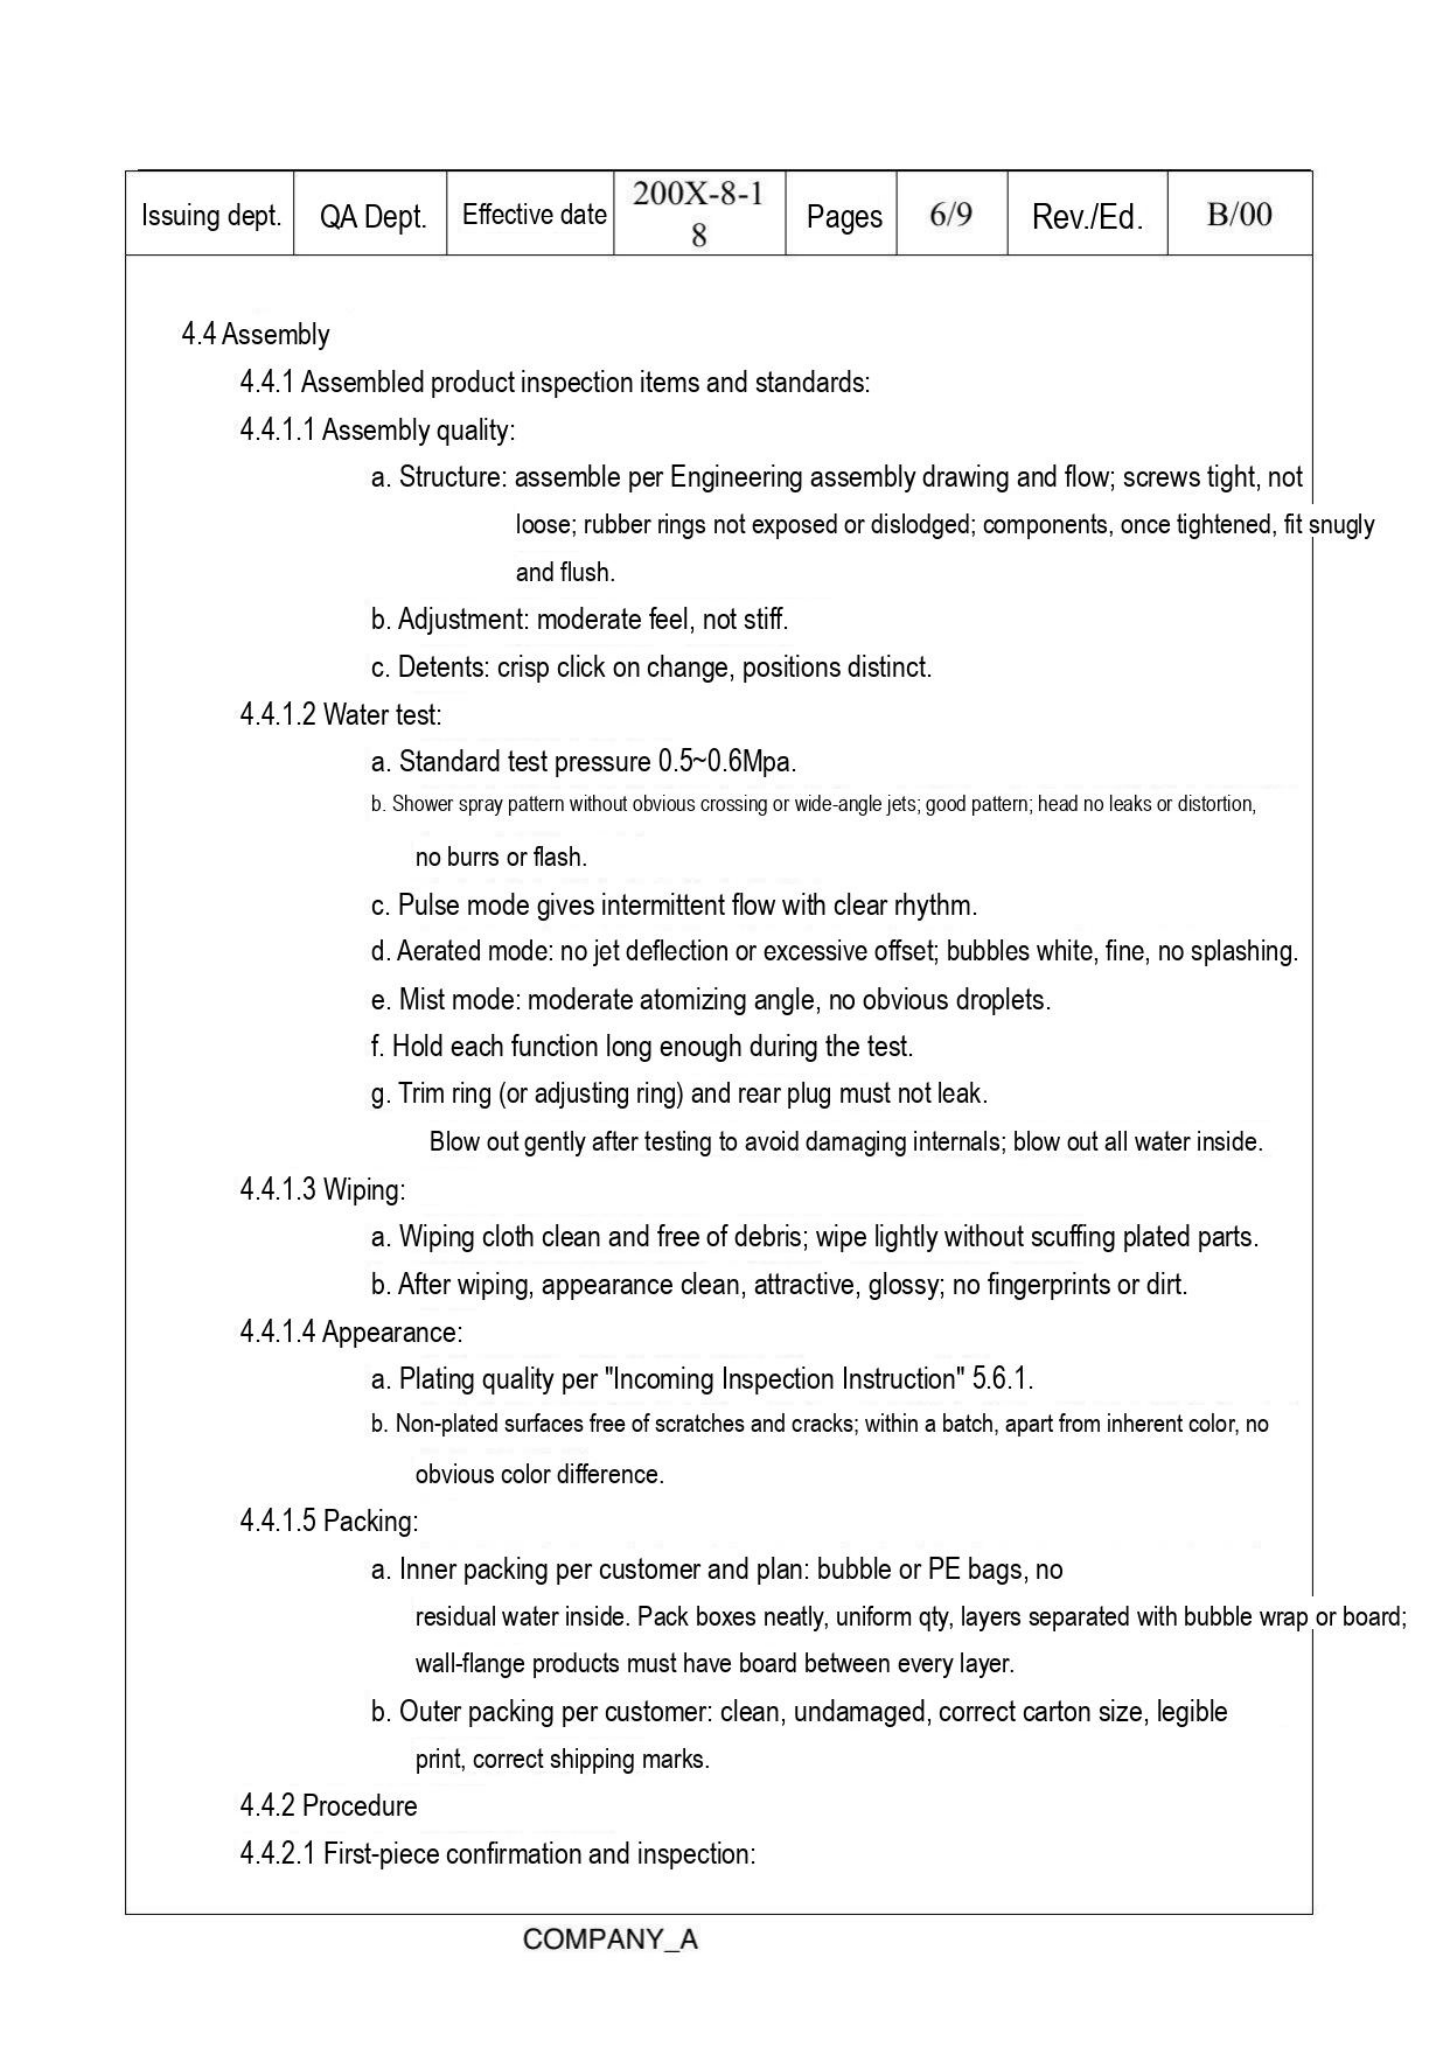| Issuing dept. | QA Dept. | Effective date | 200X-8-18 | Pages | 6/9 | Rev./Ed. | B/00 |
|---|---|---|---|---|---|---|---|

4.4 Assembly

4.4.1 Assembled product inspection items and standards:

4.4.1.1 Assembly quality:

a. Structure: assemble per Engineering assembly drawing and flow; screws tight, not loose; rubber rings not exposed or dislodged; components, once tightened, fit snugly and flush.

b. Adjustment: moderate feel, not stiff.

c. Detents: crisp click on change, positions distinct.

4.4.1.2 Water test:

a. Standard test pressure 0.5~0.6Mpa.

b. Shower spray pattern without obvious crossing or wide-angle jets; good pattern; head no leaks or distortion, no burrs or flash.

c. Pulse mode gives intermittent flow with clear rhythm.

d. Aerated mode: no jet deflection or excessive offset; bubbles white, fine, no splashing.

e. Mist mode: moderate atomizing angle, no obvious droplets.

f. Hold each function long enough during the test.

g. Trim ring (or adjusting ring) and rear plug must not leak.

Blow out gently after testing to avoid damaging internals; blow out all water inside.

4.4.1.3 Wiping:

a. Wiping cloth clean and free of debris; wipe lightly without scuffing plated parts.

b. After wiping, appearance clean, attractive, glossy; no fingerprints or dirt.

4.4.1.4 Appearance:

a. Plating quality per "Incoming Inspection Instruction" 5.6.1.

b. Non-plated surfaces free of scratches and cracks; within a batch, apart from inherent color, no obvious color difference.

4.4.1.5 Packing:

a. Inner packing per customer and plan: bubble or PE bags, no residual water inside. Pack boxes neatly, uniform qty, layers separated with bubble wrap or board; wall-flange products must have board between every layer.

b. Outer packing per customer: clean, undamaged, correct carton size, legible print, correct shipping marks.

4.4.2 Procedure

4.4.2.1 First-piece confirmation and inspection:

COMPANY_A
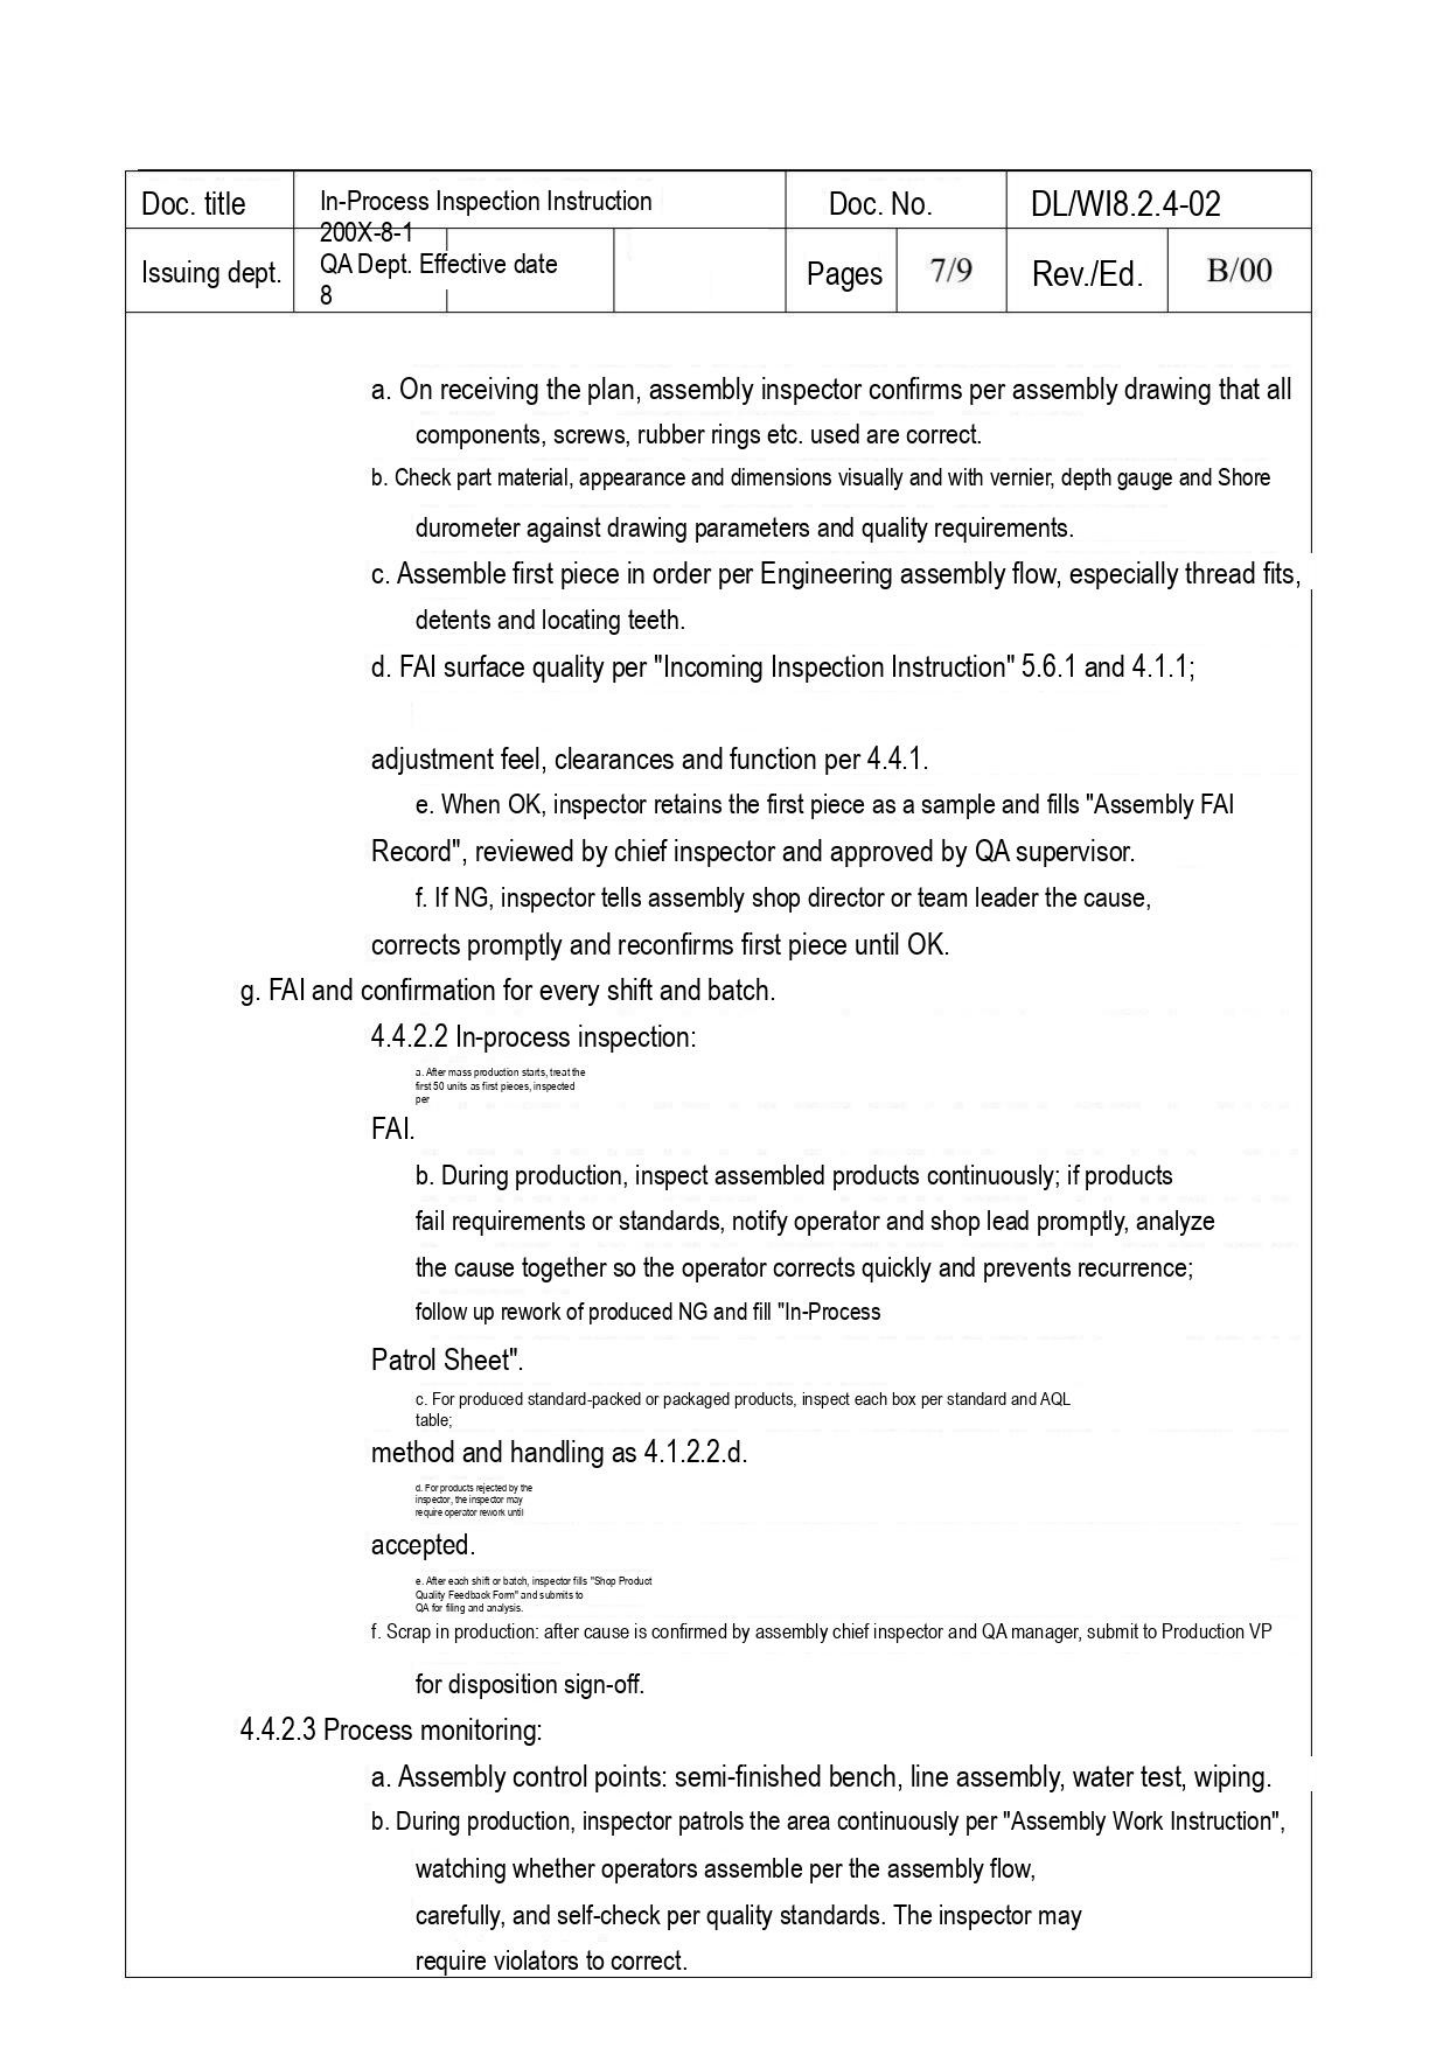| Doc. title | In-Process Inspection Instruction | | Doc. No. | DL/WI8.2.4-02 | |
|---|---|---|---|---|---|
| Issuing dept. | 200X-8-1 QA Dept. Effective date 8 | | Pages | 7/9 | Rev./Ed. | B/00 |

a. On receiving the plan, assembly inspector confirms per assembly drawing that all components, screws, rubber rings etc. used are correct.

b. Check part material, appearance and dimensions visually and with vernier, depth gauge and Shore durometer against drawing parameters and quality requirements.

c. Assemble first piece in order per Engineering assembly flow, especially thread fits, detents and locating teeth.

d. FAI surface quality per "Incoming Inspection Instruction" 5.6.1 and 4.1.1;

adjustment feel, clearances and function per 4.4.1.

e. When OK, inspector retains the first piece as a sample and fills "Assembly FAI Record", reviewed by chief inspector and approved by QA supervisor.

f. If NG, inspector tells assembly shop director or team leader the cause, corrects promptly and reconfirms first piece until OK.

g. FAI and confirmation for every shift and batch.

4.4.2.2 In-process inspection:

a. After mass production starts, treat the first 50 units as first pieces, inspected per FAI.

b. During production, inspect assembled products continuously; if products fail requirements or standards, notify operator and shop lead promptly, analyze the cause together so the operator corrects quickly and prevents recurrence; follow up rework of produced NG and fill "In-Process Patrol Sheet".

c. For produced standard-packed or packaged products, inspect each box per standard and AQL table; method and handling as 4.1.2.2.d.

d. For products rejected by the inspector, the inspector may require operator rework until accepted.

e. After each shift or batch, inspector fills "Shop Product Quality Feedback Form" and submits to QA for filing and analysis.

f. Scrap in production: after cause is confirmed by assembly chief inspector and QA manager, submit to Production VP for disposition sign-off.

4.4.2.3 Process monitoring:

a. Assembly control points: semi-finished bench, line assembly, water test, wiping.

b. During production, inspector patrols the area continuously per "Assembly Work Instruction", watching whether operators assemble per the assembly flow, carefully, and self-check per quality standards. The inspector may require violators to correct.
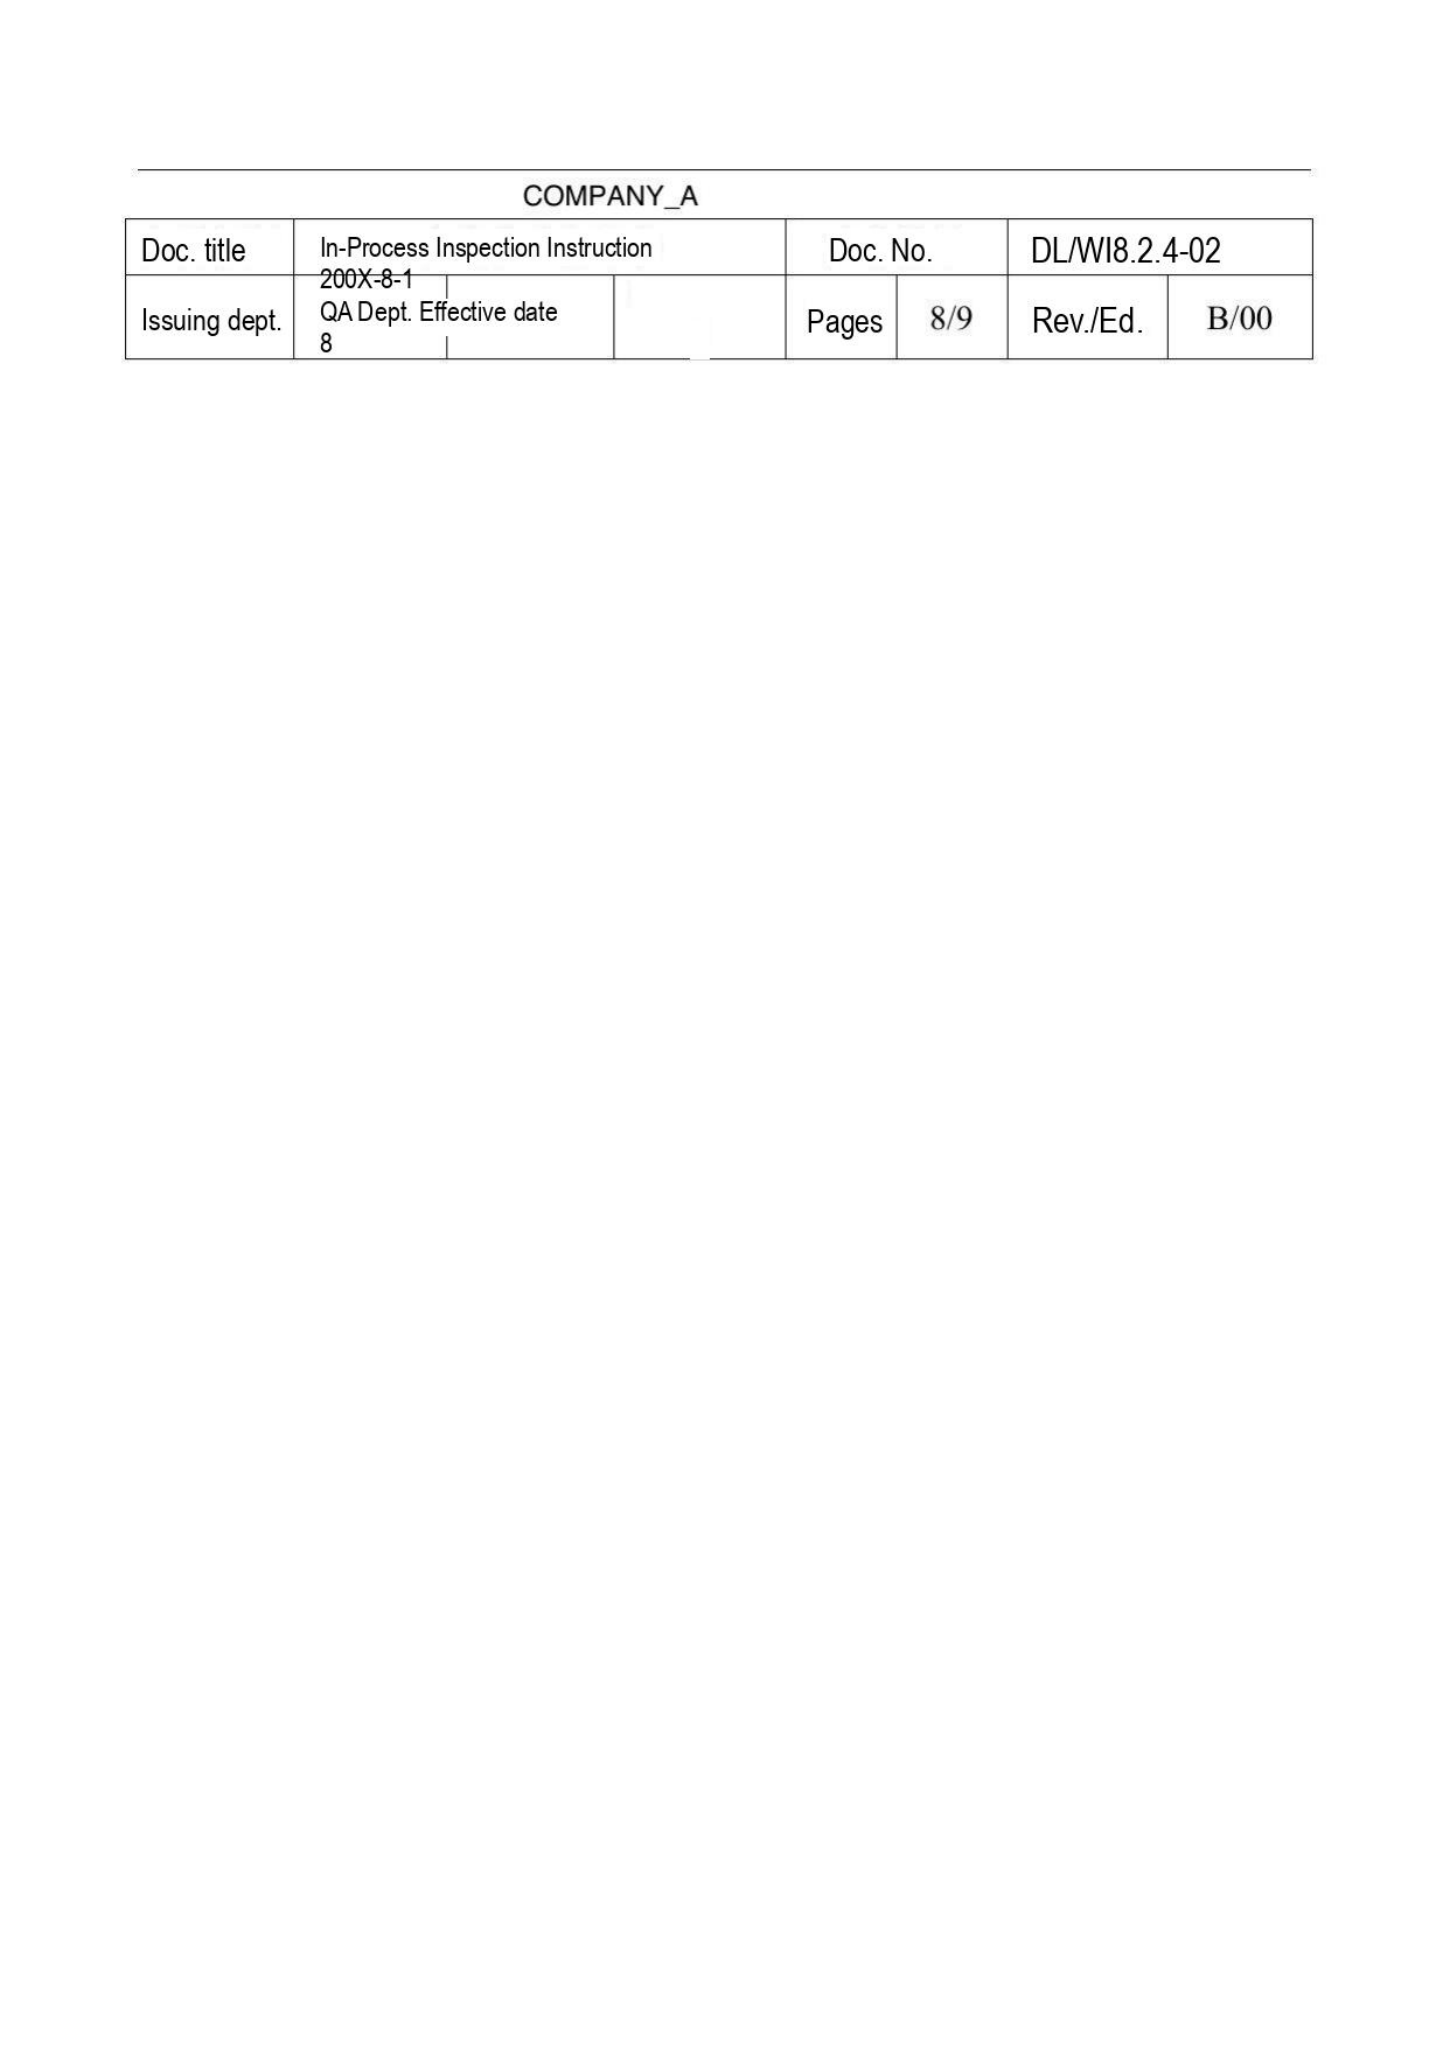COMPANY_A

| Doc. title | In-Process Inspection Instruction | | Doc. No. | | DL/WI8.2.4-02 | |
|---|---|---|---|---|---|---|
| Issuing dept. | 200X-8-1<br>QA Dept. Effective date<br>8 | | Pages | 8/9 | Rev./Ed. | B/00 |
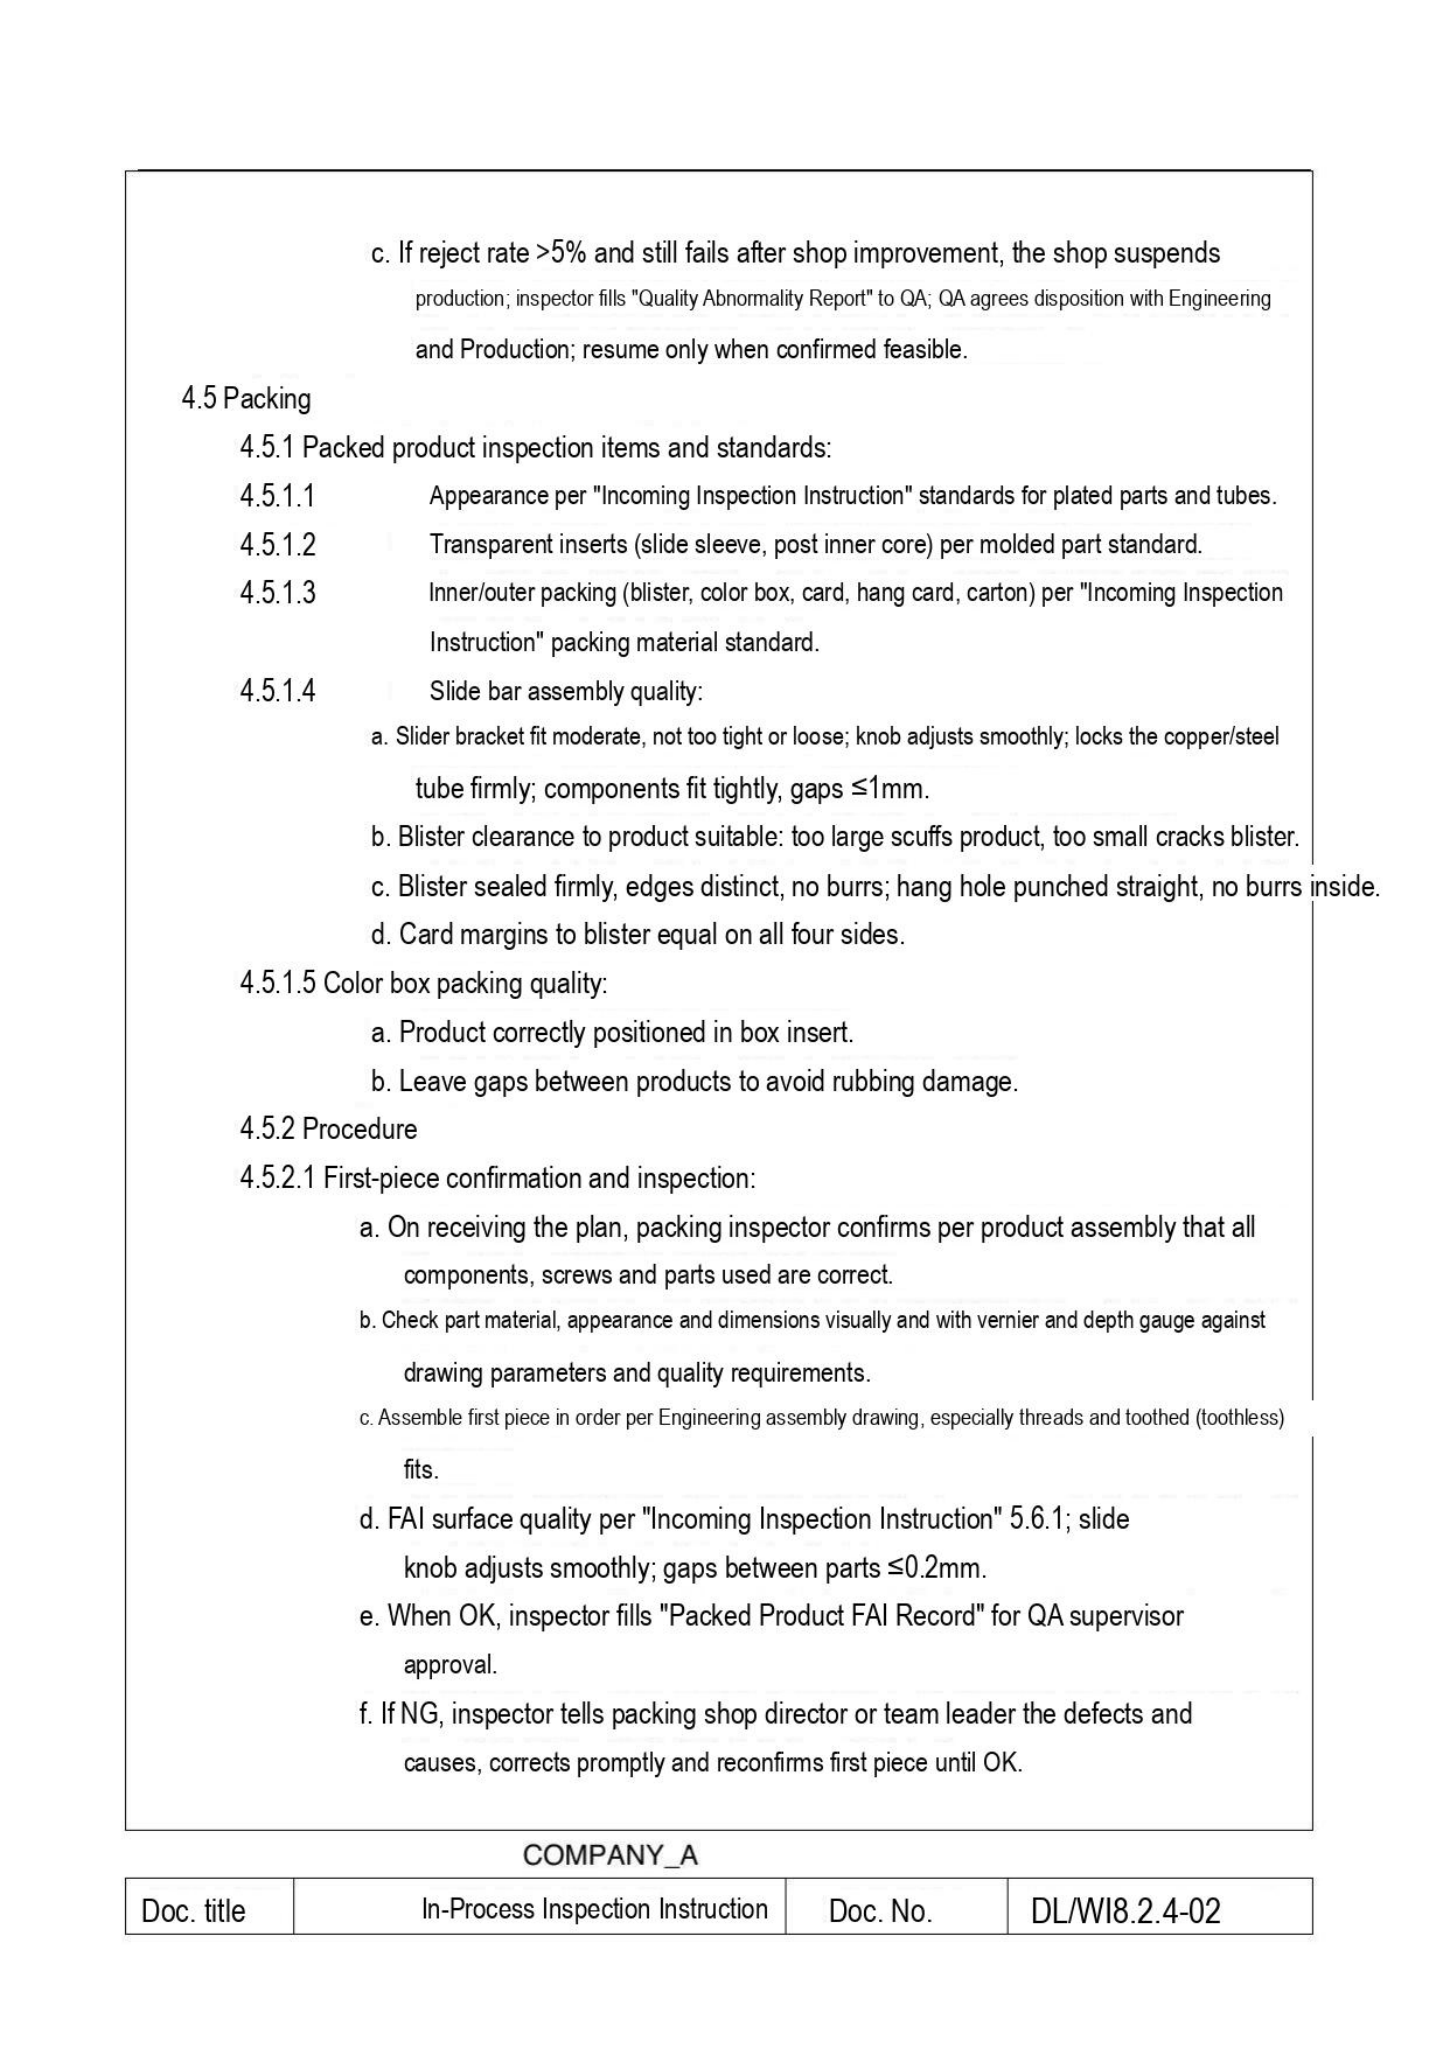c. If reject rate >5% and still fails after shop improvement, the shop suspends production; inspector fills "Quality Abnormality Report" to QA; QA agrees disposition with Engineering and Production; resume only when confirmed feasible.

4.5 Packing

4.5.1 Packed product inspection items and standards:

4.5.1.1 Appearance per "Incoming Inspection Instruction" standards for plated parts and tubes.

4.5.1.2 Transparent inserts (slide sleeve, post inner core) per molded part standard.

4.5.1.3 Inner/outer packing (blister, color box, card, hang card, carton) per "Incoming Inspection Instruction" packing material standard.

4.5.1.4 Slide bar assembly quality:

a. Slider bracket fit moderate, not too tight or loose; knob adjusts smoothly; locks the copper/steel tube firmly; components fit tightly, gaps ≤1mm.

b. Blister clearance to product suitable: too large scuffs product, too small cracks blister.

c. Blister sealed firmly, edges distinct, no burrs; hang hole punched straight, no burrs inside.

d. Card margins to blister equal on all four sides.

4.5.1.5 Color box packing quality:

a. Product correctly positioned in box insert.

b. Leave gaps between products to avoid rubbing damage.

4.5.2 Procedure

4.5.2.1 First-piece confirmation and inspection:

a. On receiving the plan, packing inspector confirms per product assembly that all components, screws and parts used are correct.

b. Check part material, appearance and dimensions visually and with vernier and depth gauge against drawing parameters and quality requirements.

c. Assemble first piece in order per Engineering assembly drawing, especially threads and toothed (toothless) fits.

d. FAI surface quality per "Incoming Inspection Instruction" 5.6.1; slide knob adjusts smoothly; gaps between parts ≤0.2mm.

e. When OK, inspector fills "Packed Product FAI Record" for QA supervisor approval.

f. If NG, inspector tells packing shop director or team leader the defects and causes, corrects promptly and reconfirms first piece until OK.

COMPANY_A

| Doc. title | In-Process Inspection Instruction | Doc. No. | DL/WI8.2.4-02 |
|---|---|---|---|
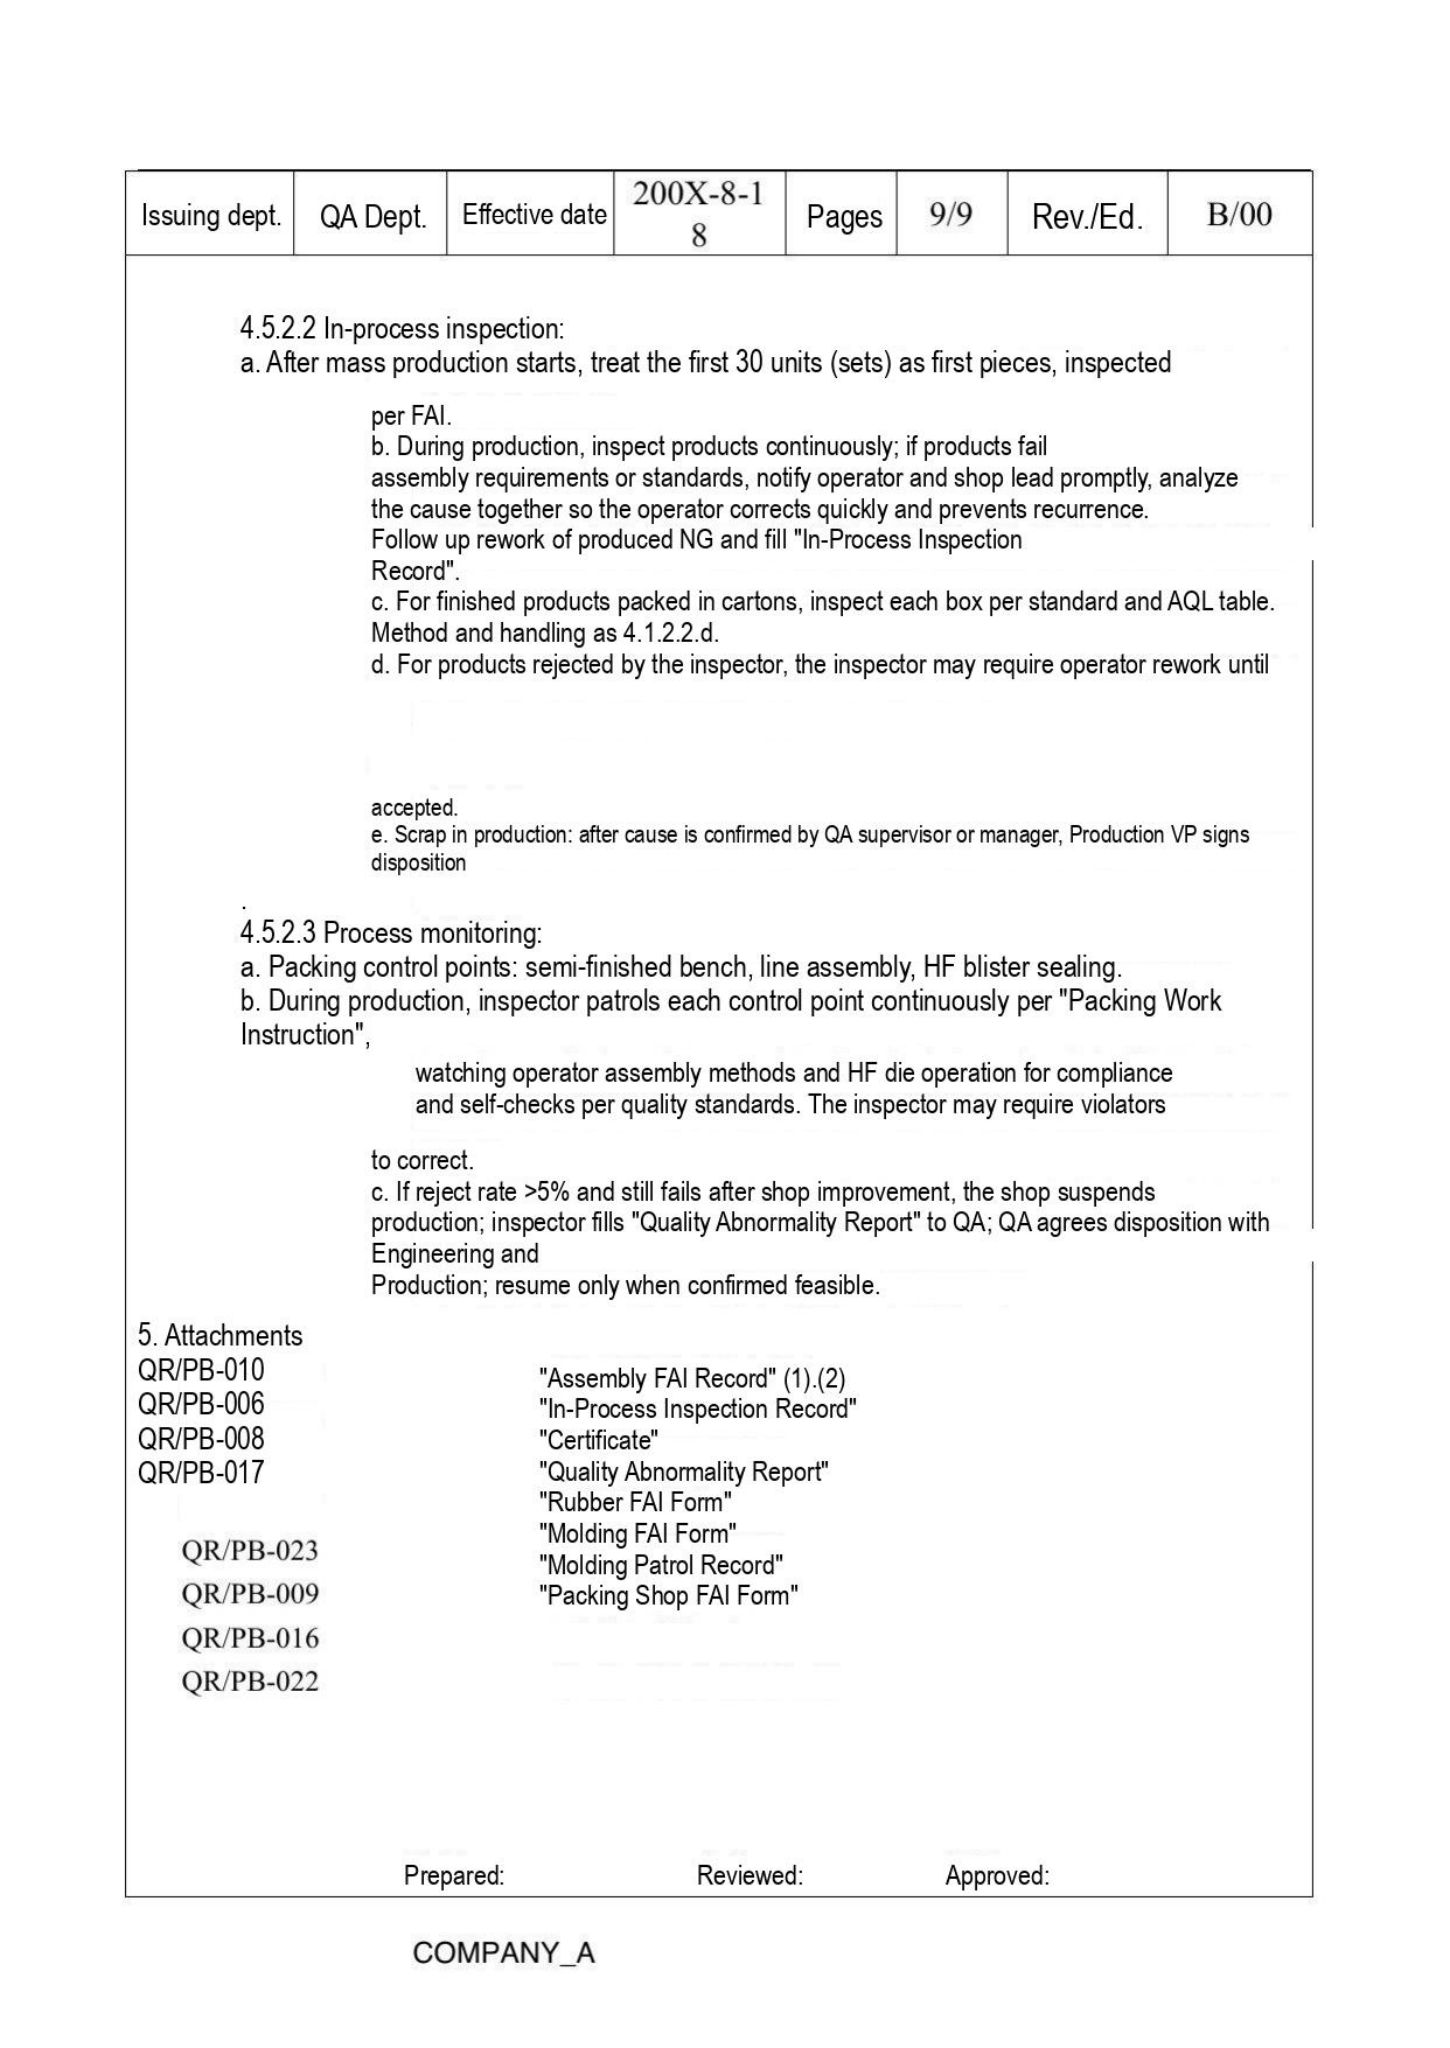| Issuing dept. | QA Dept. | Effective date | 200X-8-18 | Pages | 9/9 | Rev./Ed. | B/00 |
|---|---|---|---|---|---|---|---|

4.5.2.2 In-process inspection:
a. After mass production starts, treat the first 30 units (sets) as first pieces, inspected per FAI.
b. During production, inspect products continuously; if products fail assembly requirements or standards, notify operator and shop lead promptly, analyze the cause together so the operator corrects quickly and prevents recurrence.
Follow up rework of produced NG and fill "In-Process Inspection Record".
c. For finished products packed in cartons, inspect each box per standard and AQL table. Method and handling as 4.1.2.2.d.
d. For products rejected by the inspector, the inspector may require operator rework until accepted.
e. Scrap in production: after cause is confirmed by QA supervisor or manager, Production VP signs disposition
.
4.5.2.3 Process monitoring:
a. Packing control points: semi-finished bench, line assembly, HF blister sealing.
b. During production, inspector patrols each control point continuously per "Packing Work Instruction", watching operator assembly methods and HF die operation for compliance and self-checks per quality standards. The inspector may require violators to correct.
c. If reject rate >5% and still fails after shop improvement, the shop suspends production; inspector fills "Quality Abnormality Report" to QA; QA agrees disposition with Engineering and Production; resume only when confirmed feasible.

5. Attachments
QR/PB-010 "Assembly FAI Record" (1).(2)
QR/PB-006 "In-Process Inspection Record"
QR/PB-008 "Certificate"
QR/PB-017 "Quality Abnormality Report"
QR/PB-023 "Rubber FAI Form"
QR/PB-009 "Molding FAI Form"
QR/PB-016 "Molding Patrol Record"
QR/PB-022 "Packing Shop FAI Form"

Prepared: Reviewed: Approved:

COMPANY_A
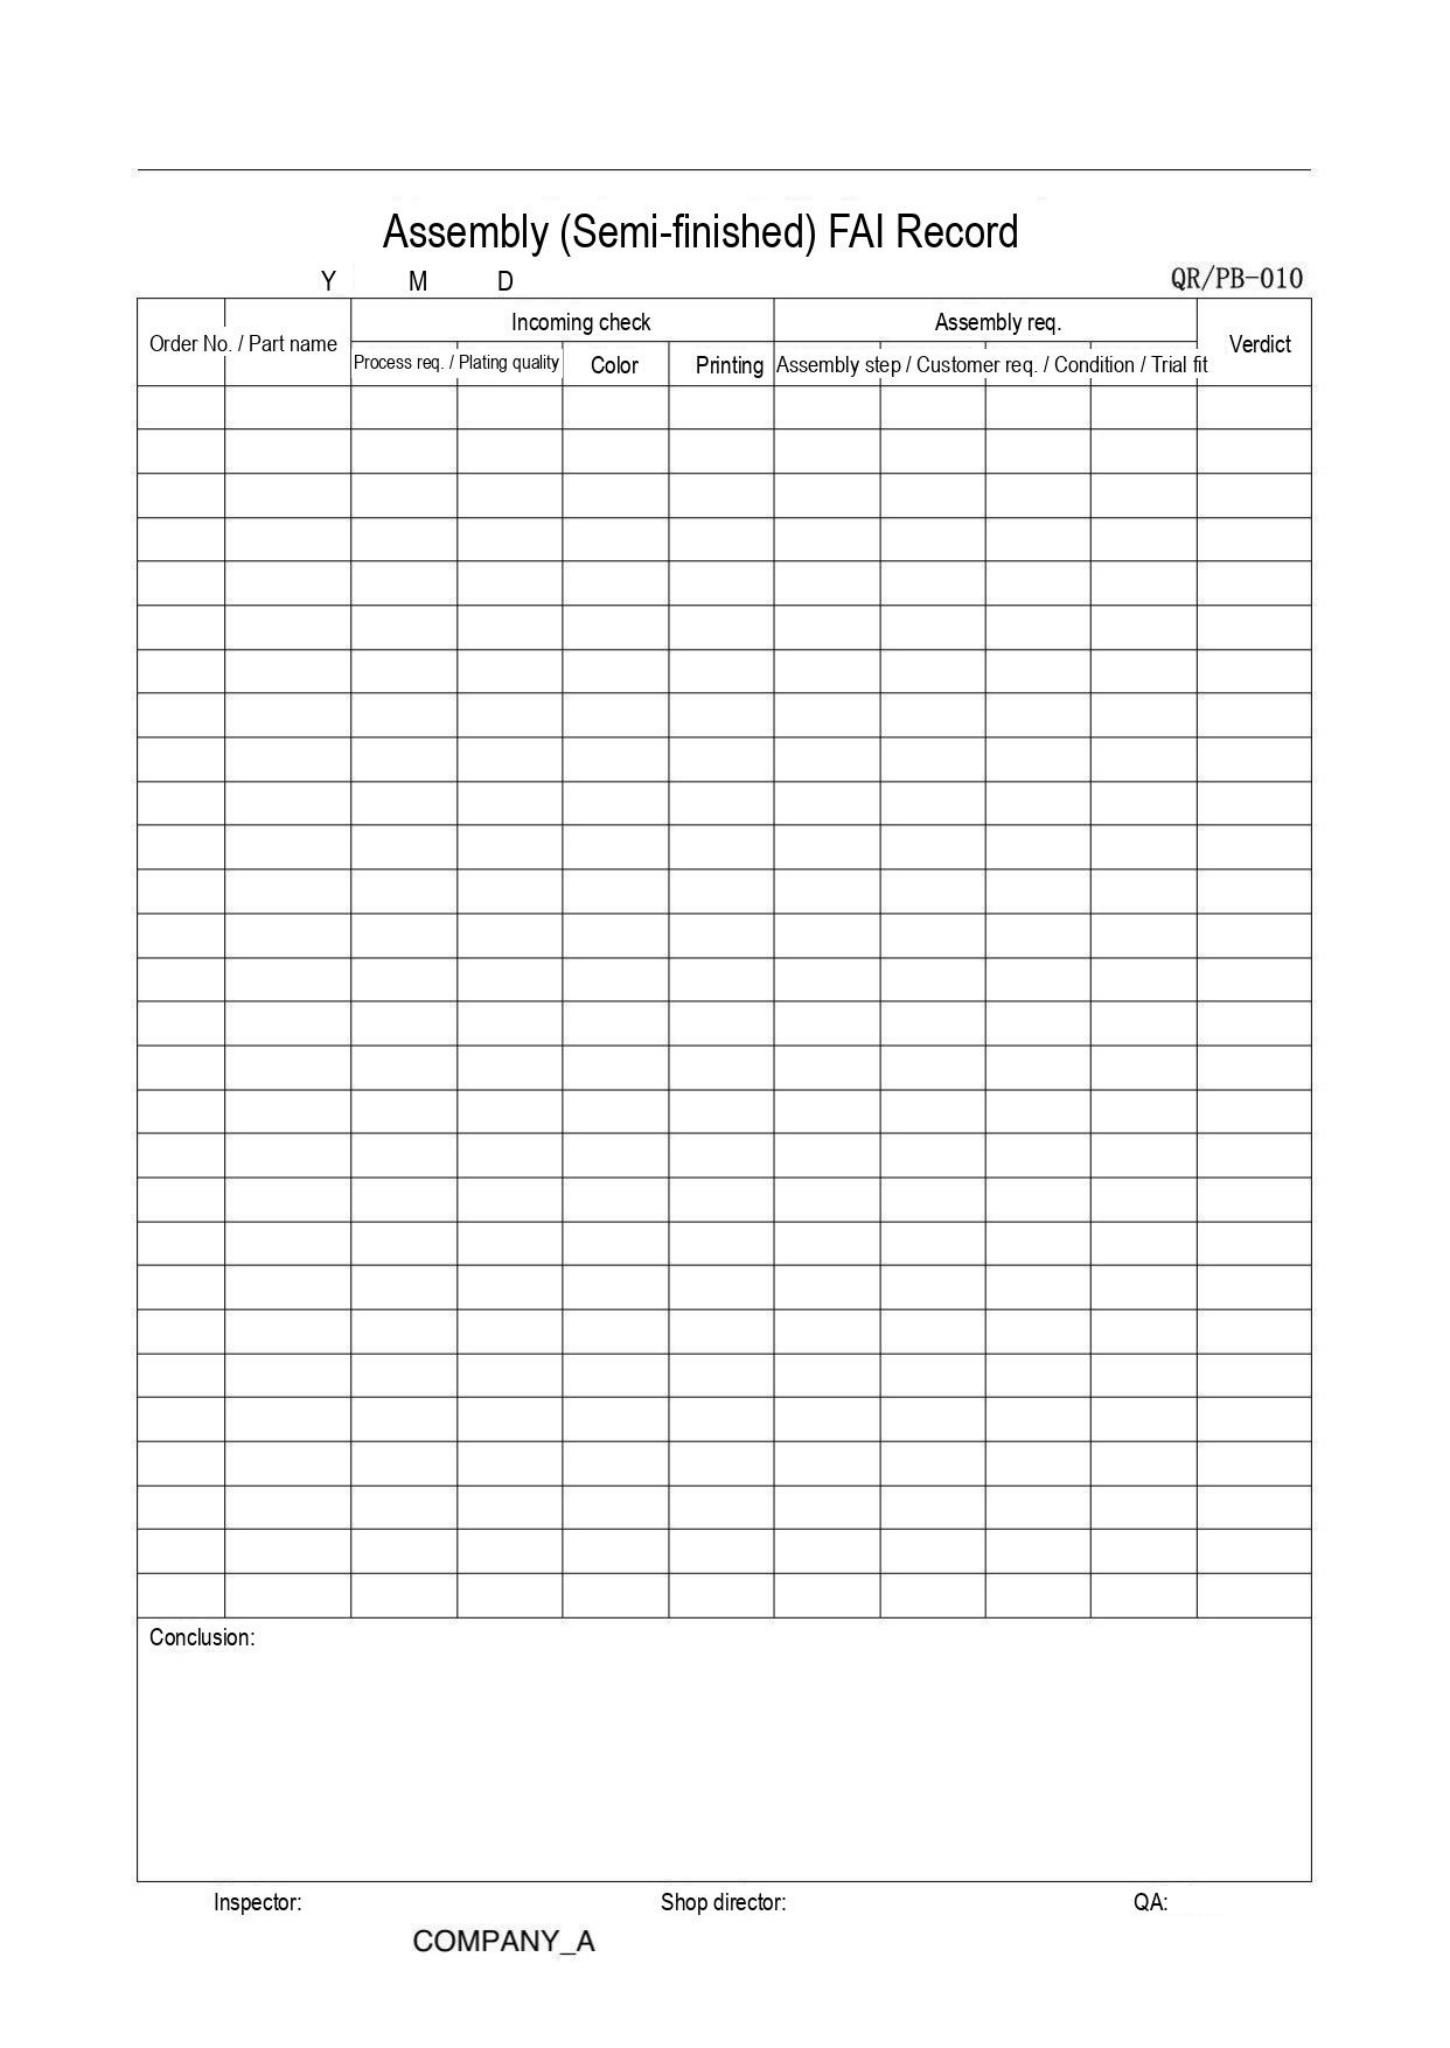Assembly (Semi-finished) FAI Record

Y M D QR/PB-010

| Order No. / Part name | | Incoming check | | | | Assembly req. | | | | Verdict |
|---|---|---|---|---|---|---|---|---|---|---|
| | | Process req. / Plating quality | | Color | Printing | Assembly step / Customer req. / Condition / Trial fit | | | | |
| | | | | | | | | | | |
| | | | | | | | | | | |
| | | | | | | | | | | |
| | | | | | | | | | | |
| | | | | | | | | | | |
| | | | | | | | | | | |
| | | | | | | | | | | |
| | | | | | | | | | | |
| | | | | | | | | | | |
| | | | | | | | | | | |
| | | | | | | | | | | |
| | | | | | | | | | | |
| | | | | | | | | | | |
| | | | | | | | | | | |
| | | | | | | | | | | |
| | | | | | | | | | | |
| | | | | | | | | | | |
| | | | | | | | | | | |
| | | | | | | | | | | |
| | | | | | | | | | | |
| | | | | | | | | | | |
| | | | | | | | | | | |
| | | | | | | | | | | |
| | | | | | | | | | | |
| | | | | | | | | | | |
| | | | | | | | | | | |
| | | | | | | | | | | |
| | | | | | | | | | | |

Conclusion:

Inspector: Shop director: QA:

COMPANY_A
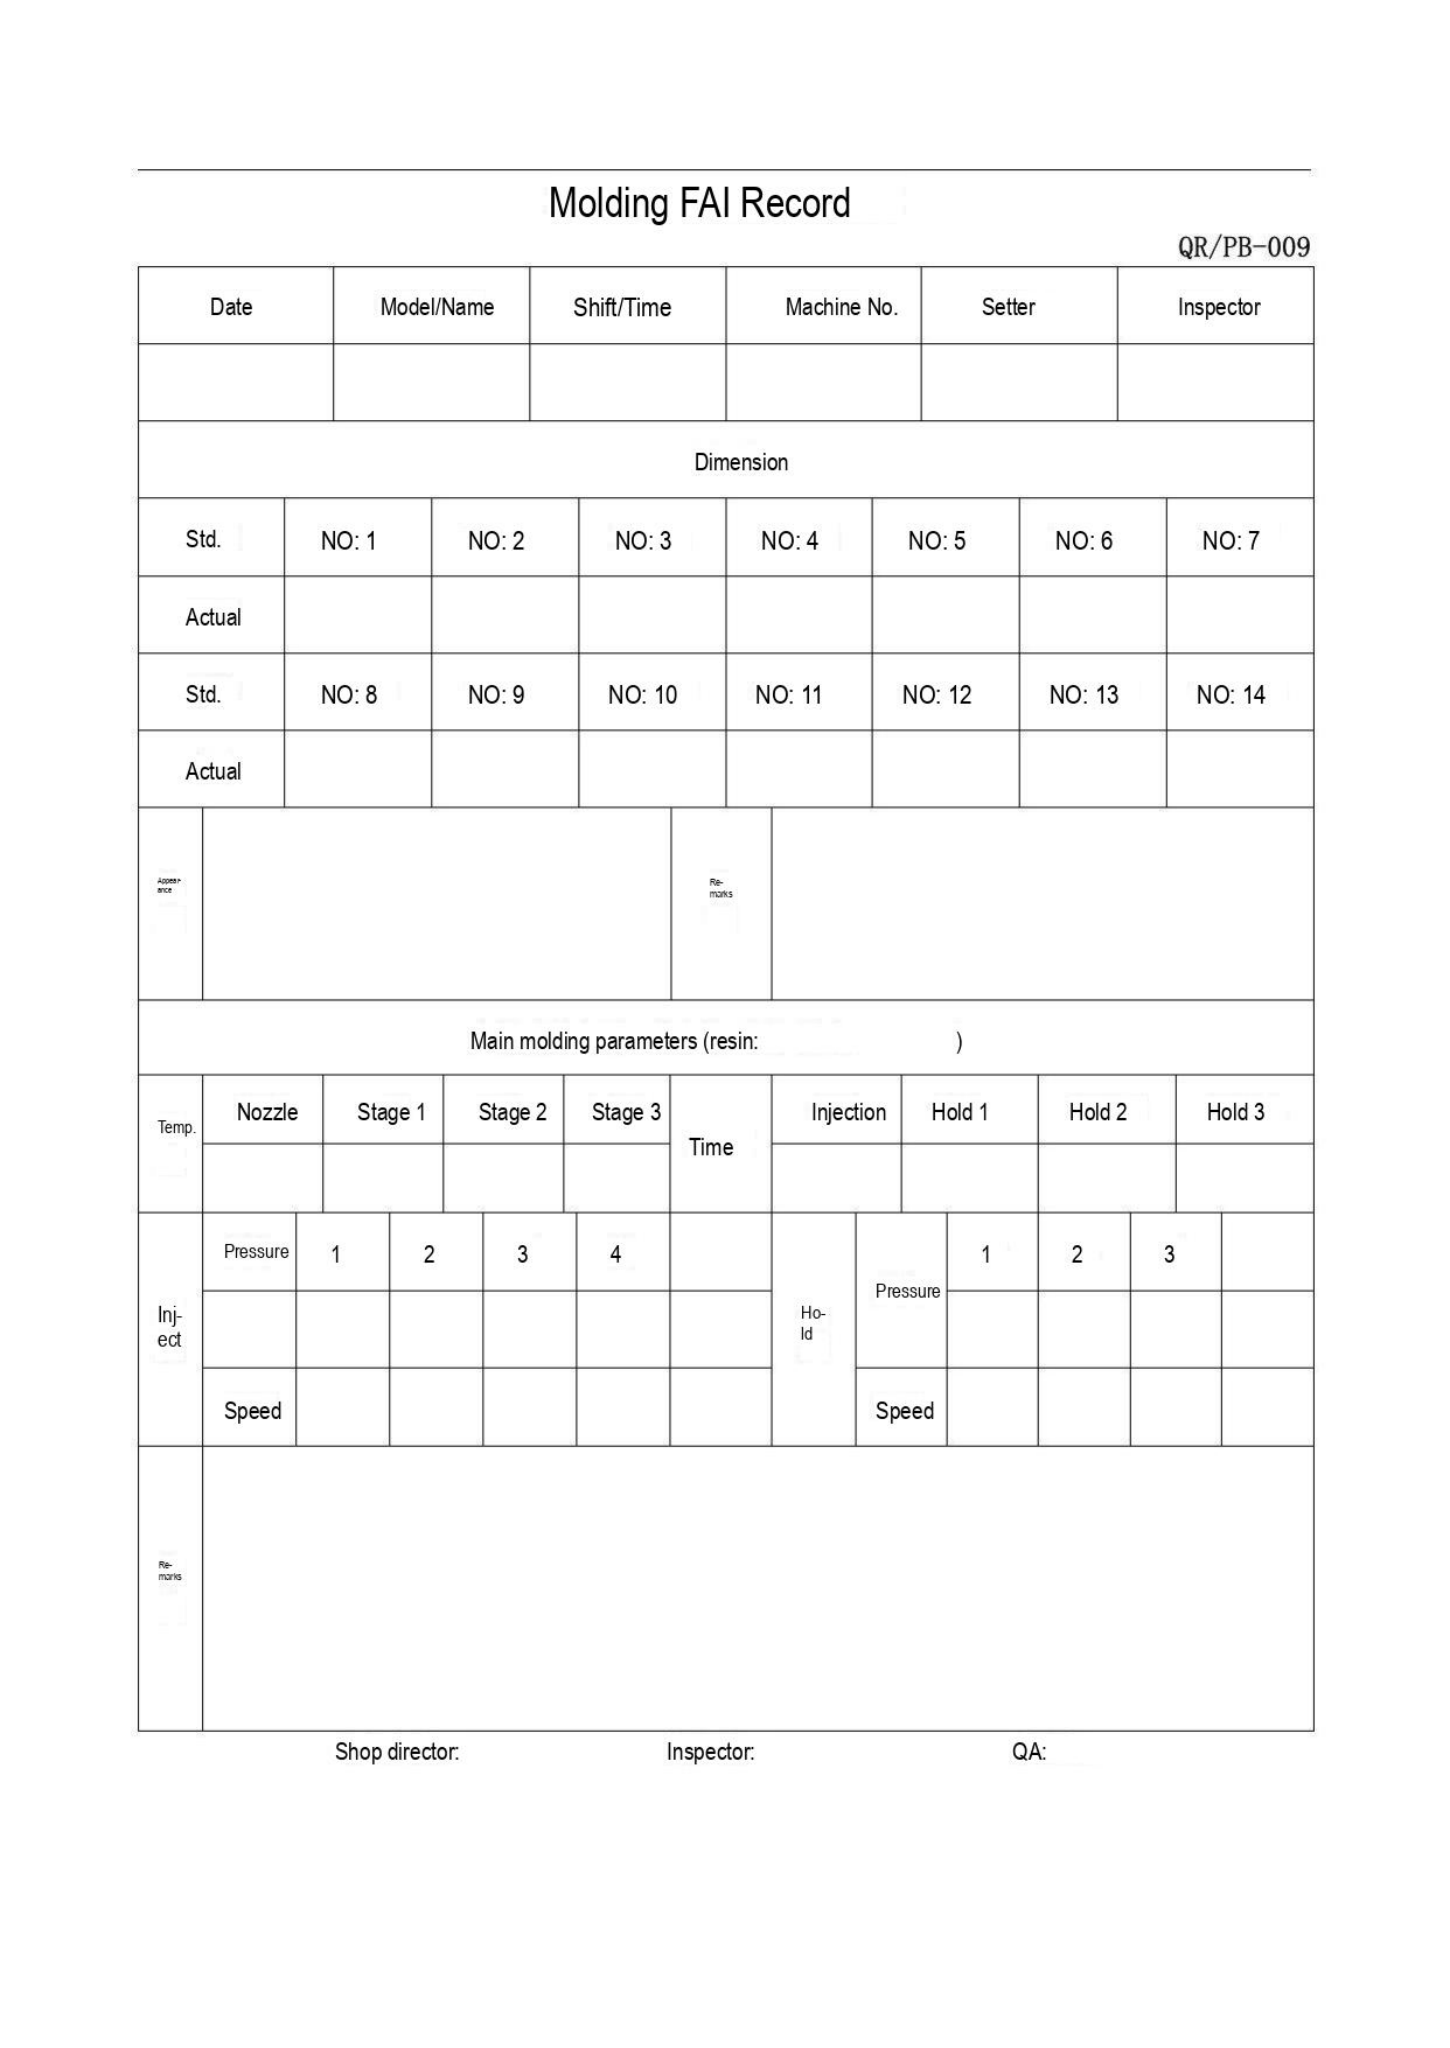Molding FAI Record

QR/PB-009

| Date | Model/Name | Shift/Time | Machine No. | Setter | Inspector |
|---|---|---|---|---|---|
| | | | | | |

| Dimension | | | | | | | |
|---|---|---|---|---|---|---|---|
| Std. | NO: 1 | NO: 2 | NO: 3 | NO: 4 | NO: 5 | NO: 6 | NO: 7 |
| Actual | | | | | | | |
| Std. | NO: 8 | NO: 9 | NO: 10 | NO: 11 | NO: 12 | NO: 13 | NO: 14 |
| Actual | | | | | | | |

| Appear-ance | | Re-marks | |
|---|---|---|---|

Main molding parameters (resin: )

| Temp. | Nozzle | Stage 1 | Stage 2 | Stage 3 | Time | Injection | Hold 1 | Hold 2 | Hold 3 |
|---|---|---|---|---|---|---|---|---|---|
| | | | | | | | | | |

| Inj-ect | Pressure | 1 | 2 | 3 | 4 | | Ho-ld | Pressure | 1 | 2 | 3 | |
|---|---|---|---|---|---|---|---|---|---|---|---|---|
| | | | | | | | | | | | | |
| | Speed | | | | | | | Speed | | | | |

| Re-marks | |
|---|---|

Shop director: Inspector: QA: